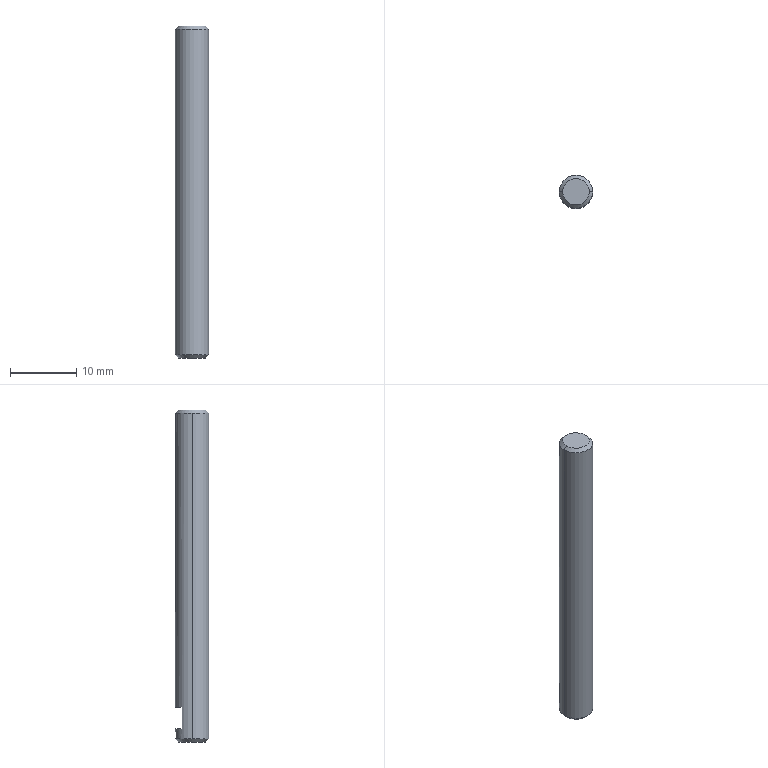Part | SolidWorks | features Chamfer 1, Extrusion 1, ICE 1 | 1 solid | 11 faces | box 5 x 5 x 50 mm | volume 969.137 mm3 | plane 5 | cone 4 | cylinder 2 | commonest cylinder face diameters 5 x2
STEP:
#1=CARTESIAN_POINT('',(2.,0.,25.));
#2=VERTEX_POINT('',#1);
#3=CARTESIAN_POINT('',(-2.,0.,25.));
#4=VERTEX_POINT('',#3);
#5=CARTESIAN_POINT('',(0.,0.,25.));
#6=DIRECTION('',(0.,0.,1.));
#7=DIRECTION('',(1.,0.,0.));
#8=AXIS2_PLACEMENT_3D('',#5,#6,#7);
#9=CIRCLE('',#8,2.);
#10=EDGE_CURVE('',#2,#4,#9,.T.);
#11=ORIENTED_EDGE('',*,*,#10,.F.);
#12=CARTESIAN_POINT('',(2.5,0.,24.5));
#13=VERTEX_POINT('',#12);
#14=CARTESIAN_POINT('',(2.,0.,25.));
#15=DIRECTION('',(0.7071,0.,-0.7071));
#16=VECTOR('',#15,1000.);
#17=LINE('',#14,#16);
#18=EDGE_CURVE('',#2,#13,#17,.T.);
#19=ORIENTED_EDGE('',*,*,#18,.T.);
#20=CARTESIAN_POINT('',(-2.5,0.,24.5));
#21=VERTEX_POINT('',#20);
#22=CARTESIAN_POINT('',(0.,0.,24.5));
#23=DIRECTION('',(0.,0.,-1.));
#24=DIRECTION('',(1.,0.,0.));
#25=AXIS2_PLACEMENT_3D('',#22,#23,#24);
#26=CIRCLE('',#25,2.5);
#27=EDGE_CURVE('',#21,#13,#26,.T.);
#28=ORIENTED_EDGE('',*,*,#27,.F.);
#29=CARTESIAN_POINT('',(-2.,0.,25.));
#30=DIRECTION('',(-0.7071,0.,-0.7071));
#31=VECTOR('',#30,1000.);
#32=LINE('',#29,#31);
#33=EDGE_CURVE('',#4,#21,#32,.T.);
#34=ORIENTED_EDGE('',*,*,#33,.F.);
#35=EDGE_LOOP('',(#11,#19,#28,#34));
#36=FACE_OUTER_BOUND('',#35,.T.);
#37=CARTESIAN_POINT('',(0.,0.,25.));
#38=DIRECTION('',(0.,0.,-1.));
#39=DIRECTION('',(-1.,0.,0.));
#40=AXIS2_PLACEMENT_3D('',#37,#38,#39);
#41=CONICAL_SURFACE('',#40,2.,0.7854);
#42=ADVANCED_FACE('',(#36),#41,.T.);
#43=CARTESIAN_POINT('',(-2.,0.,-25.));
#44=VERTEX_POINT('',#43);
#45=CARTESIAN_POINT('',(2.,0.,-25.));
#46=VERTEX_POINT('',#45);
#47=CARTESIAN_POINT('',(0.,0.,-25.));
#48=DIRECTION('',(0.,0.,-1.));
#49=DIRECTION('',(1.,0.,0.));
#50=AXIS2_PLACEMENT_3D('',#47,#48,#49);
#51=CIRCLE('',#50,2.);
#52=EDGE_CURVE('',#44,#46,#51,.T.);
#53=ORIENTED_EDGE('',*,*,#52,.F.);
#54=CARTESIAN_POINT('',(-2.5,0.,-24.5));
#55=VERTEX_POINT('',#54);
#56=CARTESIAN_POINT('',(-2.5,0.,-24.5));
#57=DIRECTION('',(-0.7071,0.,0.7071));
#58=VECTOR('',#57,1000.);
#59=LINE('',#56,#58);
#60=EDGE_CURVE('',#44,#55,#59,.T.);
#61=ORIENTED_EDGE('',*,*,#60,.T.);
#62=CARTESIAN_POINT('',(2.5,0.,-24.5));
#63=VERTEX_POINT('',#62);
#64=CARTESIAN_POINT('',(0.,0.,-24.5));
#65=DIRECTION('',(0.,0.,1.));
#66=DIRECTION('',(1.,0.,0.));
#67=AXIS2_PLACEMENT_3D('',#64,#65,#66);
#68=CIRCLE('',#67,2.5);
#69=EDGE_CURVE('',#63,#55,#68,.T.);
#70=ORIENTED_EDGE('',*,*,#69,.F.);
#71=CARTESIAN_POINT('',(2.5,0.,-24.5));
#72=DIRECTION('',(0.7071,0.,0.7071));
#73=VECTOR('',#72,1000.);
#74=LINE('',#71,#73);
#75=EDGE_CURVE('',#46,#63,#74,.T.);
#76=ORIENTED_EDGE('',*,*,#75,.F.);
#77=EDGE_LOOP('',(#53,#61,#70,#76));
#78=FACE_OUTER_BOUND('',#77,.T.);
#79=CARTESIAN_POINT('',(0.,0.,-24.5));
#80=DIRECTION('',(0.,0.,1.));
#81=DIRECTION('',(1.,0.,0.));
#82=AXIS2_PLACEMENT_3D('',#79,#80,#81);
#83=CONICAL_SURFACE('',#82,2.5,0.7854);
#84=ADVANCED_FACE('',(#78),#83,.T.);
#85=CARTESIAN_POINT('',(-2.,1.5,-19.8));
#86=VERTEX_POINT('',#85);
#87=CARTESIAN_POINT('',(-2.,1.5,-23.));
#88=VERTEX_POINT('',#87);
#89=CARTESIAN_POINT('',(-2.,1.5,25.));
#90=DIRECTION('',(0.,0.,-1.));
#91=VECTOR('',#90,1000.);
#92=LINE('',#89,#91);
#93=EDGE_CURVE('',#86,#88,#92,.T.);
#94=ORIENTED_EDGE('',*,*,#93,.T.);
#95=CARTESIAN_POINT('',(2.,1.5,-23.));
#96=VERTEX_POINT('',#95);
#97=CARTESIAN_POINT('',(0.,0.,-23.));
#98=DIRECTION('',(0.,0.,-1.));
#99=DIRECTION('',(-1.,0.,0.));
#100=AXIS2_PLACEMENT_3D('',#97,#98,#99);
#101=CIRCLE('',#100,2.5);
#102=EDGE_CURVE('',#88,#96,#101,.T.);
#103=ORIENTED_EDGE('',*,*,#102,.T.);
#104=CARTESIAN_POINT('',(2.,1.5,-19.8));
#105=VERTEX_POINT('',#104);
#106=CARTESIAN_POINT('',(2.,1.5,25.));
#107=DIRECTION('',(0.,0.,1.));
#108=VECTOR('',#107,1000.);
#109=LINE('',#106,#108);
#110=EDGE_CURVE('',#96,#105,#109,.T.);
#111=ORIENTED_EDGE('',*,*,#110,.T.);
#112=CARTESIAN_POINT('',(0.,0.,-19.8));
#113=DIRECTION('',(0.,0.,1.));
#114=DIRECTION('',(0.,-1.,0.));
#115=AXIS2_PLACEMENT_3D('',#112,#113,#114);
#116=CIRCLE('',#115,2.5);
#117=EDGE_CURVE('',#105,#86,#116,.T.);
#118=ORIENTED_EDGE('',*,*,#117,.T.);
#119=EDGE_LOOP('',(#94,#103,#111,#118));
#120=FACE_BOUND('',#119,.T.);
#121=ORIENTED_EDGE('',*,*,#27,.T.);
#122=CARTESIAN_POINT('',(2.5,0.,25.));
#123=DIRECTION('',(0.,0.,-1.));
#124=VECTOR('',#123,1000.);
#125=LINE('',#122,#124);
#126=EDGE_CURVE('',#13,#63,#125,.T.);
#127=ORIENTED_EDGE('',*,*,#126,.T.);
#128=ORIENTED_EDGE('',*,*,#69,.T.);
#129=CARTESIAN_POINT('',(-2.5,0.,25.));
#130=DIRECTION('',(0.,0.,-1.));
#131=VECTOR('',#130,1000.);
#132=LINE('',#129,#131);
#133=EDGE_CURVE('',#21,#55,#132,.T.);
#134=ORIENTED_EDGE('',*,*,#133,.F.);
#135=EDGE_LOOP('',(#121,#127,#128,#134));
#136=FACE_OUTER_BOUND('',#135,.T.);
#137=CARTESIAN_POINT('',(0.,0.,25.));
#138=DIRECTION('',(0.,0.,-1.));
#139=DIRECTION('',(-1.,0.,0.));
#140=AXIS2_PLACEMENT_3D('',#137,#138,#139);
#141=CYLINDRICAL_SURFACE('',#140,2.5);
#142=ADVANCED_FACE('',(#120,#136),#141,.T.);
#143=ORIENTED_EDGE('',*,*,#126,.F.);
#144=CARTESIAN_POINT('',(0.,0.,24.5));
#145=DIRECTION('',(0.,0.,-1.));
#146=DIRECTION('',(1.,0.,0.));
#147=AXIS2_PLACEMENT_3D('',#144,#145,#146);
#148=CIRCLE('',#147,2.5);
#149=EDGE_CURVE('',#13,#21,#148,.T.);
#150=ORIENTED_EDGE('',*,*,#149,.T.);
#151=ORIENTED_EDGE('',*,*,#133,.T.);
#152=CARTESIAN_POINT('',(0.,0.,-24.5));
#153=DIRECTION('',(0.,0.,1.));
#154=DIRECTION('',(1.,0.,0.));
#155=AXIS2_PLACEMENT_3D('',#152,#153,#154);
#156=CIRCLE('',#155,2.5);
#157=EDGE_CURVE('',#55,#63,#156,.T.);
#158=ORIENTED_EDGE('',*,*,#157,.T.);
#159=EDGE_LOOP('',(#143,#150,#151,#158));
#160=FACE_OUTER_BOUND('',#159,.T.);
#161=CARTESIAN_POINT('',(0.,0.,25.));
#162=DIRECTION('',(0.,0.,-1.));
#163=DIRECTION('',(-1.,0.,0.));
#164=AXIS2_PLACEMENT_3D('',#161,#162,#163);
#165=CYLINDRICAL_SURFACE('',#164,2.5);
#166=ADVANCED_FACE('',(#160),#165,.T.);
#167=CARTESIAN_POINT('',(0.,0.,25.));
#168=DIRECTION('',(0.,0.,1.));
#169=DIRECTION('',(1.,0.,0.));
#170=AXIS2_PLACEMENT_3D('',#167,#168,#169);
#171=CIRCLE('',#170,2.);
#172=EDGE_CURVE('',#4,#2,#171,.T.);
#173=ORIENTED_EDGE('',*,*,#172,.T.);
#174=ORIENTED_EDGE('',*,*,#10,.T.);
#175=EDGE_LOOP('',(#173,#174));
#176=FACE_OUTER_BOUND('',#175,.T.);
#177=CARTESIAN_POINT('',(0.,0.,25.));
#178=DIRECTION('',(0.,0.,1.));
#179=DIRECTION('',(1.,0.,0.));
#180=AXIS2_PLACEMENT_3D('',#177,#178,#179);
#181=PLANE('',#180);
#182=ADVANCED_FACE('',(#176),#181,.T.);
#183=CARTESIAN_POINT('',(0.,0.,-25.));
#184=DIRECTION('',(0.,0.,-1.));
#185=DIRECTION('',(1.,0.,0.));
#186=AXIS2_PLACEMENT_3D('',#183,#184,#185);
#187=CIRCLE('',#186,2.);
#188=EDGE_CURVE('',#46,#44,#187,.T.);
#189=ORIENTED_EDGE('',*,*,#188,.T.);
#190=ORIENTED_EDGE('',*,*,#52,.T.);
#191=EDGE_LOOP('',(#189,#190));
#192=FACE_OUTER_BOUND('',#191,.T.);
#193=CARTESIAN_POINT('',(0.,0.,-25.));
#194=DIRECTION('',(0.,0.,1.));
#195=DIRECTION('',(1.,0.,0.));
#196=AXIS2_PLACEMENT_3D('',#193,#194,#195);
#197=PLANE('',#196);
#198=ADVANCED_FACE('',(#192),#197,.F.);
#199=ORIENTED_EDGE('',*,*,#60,.F.);
#200=ORIENTED_EDGE('',*,*,#188,.F.);
#201=ORIENTED_EDGE('',*,*,#75,.T.);
#202=ORIENTED_EDGE('',*,*,#157,.F.);
#203=EDGE_LOOP('',(#199,#200,#201,#202));
#204=FACE_OUTER_BOUND('',#203,.T.);
#205=CARTESIAN_POINT('',(0.,0.,-24.5));
#206=DIRECTION('',(0.,0.,1.));
#207=DIRECTION('',(1.,0.,0.));
#208=AXIS2_PLACEMENT_3D('',#205,#206,#207);
#209=CONICAL_SURFACE('',#208,2.5,0.7854);
#210=ADVANCED_FACE('',(#204),#209,.T.);
#211=ORIENTED_EDGE('',*,*,#18,.F.);
#212=ORIENTED_EDGE('',*,*,#172,.F.);
#213=ORIENTED_EDGE('',*,*,#33,.T.);
#214=ORIENTED_EDGE('',*,*,#149,.F.);
#215=EDGE_LOOP('',(#211,#212,#213,#214));
#216=FACE_OUTER_BOUND('',#215,.T.);
#217=CARTESIAN_POINT('',(0.,0.,25.));
#218=DIRECTION('',(0.,0.,-1.));
#219=DIRECTION('',(-1.,0.,0.));
#220=AXIS2_PLACEMENT_3D('',#217,#218,#219);
#221=CONICAL_SURFACE('',#220,2.,0.7854);
#222=ADVANCED_FACE('',(#216),#221,.T.);
#223=CARTESIAN_POINT('',(-2.5,1.5,-23.));
#224=DIRECTION('',(1.,0.,0.));
#225=VECTOR('',#224,1000.);
#226=LINE('',#223,#225);
#227=EDGE_CURVE('',#88,#96,#226,.T.);
#228=ORIENTED_EDGE('',*,*,#227,.T.);
#229=ORIENTED_EDGE('',*,*,#102,.F.);
#230=EDGE_LOOP('',(#228,#229));
#231=FACE_OUTER_BOUND('',#230,.T.);
#232=CARTESIAN_POINT('',(-2.5,5.025,-23.));
#233=DIRECTION('',(0.,0.,-1.));
#234=DIRECTION('',(-1.,0.,0.));
#235=AXIS2_PLACEMENT_3D('',#232,#233,#234);
#236=PLANE('',#235);
#237=ADVANCED_FACE('',(#231),#236,.F.);
#238=CARTESIAN_POINT('',(-2.5,1.5,-19.8));
#239=DIRECTION('',(1.,0.,0.));
#240=VECTOR('',#239,1000.);
#241=LINE('',#238,#240);
#242=EDGE_CURVE('',#86,#105,#241,.T.);
#243=ORIENTED_EDGE('',*,*,#242,.T.);
#244=ORIENTED_EDGE('',*,*,#110,.F.);
#245=ORIENTED_EDGE('',*,*,#227,.F.);
#246=ORIENTED_EDGE('',*,*,#93,.F.);
#247=EDGE_LOOP('',(#243,#244,#245,#246));
#248=FACE_OUTER_BOUND('',#247,.T.);
#249=CARTESIAN_POINT('',(-2.5,1.5,-23.));
#250=DIRECTION('',(0.,-1.,0.));
#251=DIRECTION('',(0.,0.,-1.));
#252=AXIS2_PLACEMENT_3D('',#249,#250,#251);
#253=PLANE('',#252);
#254=ADVANCED_FACE('',(#248),#253,.F.);
#255=ORIENTED_EDGE('',*,*,#242,.F.);
#256=ORIENTED_EDGE('',*,*,#117,.F.);
#257=EDGE_LOOP('',(#255,#256));
#258=FACE_OUTER_BOUND('',#257,.T.);
#259=CARTESIAN_POINT('',(-2.5,5.025,-19.8));
#260=DIRECTION('',(0.,0.,1.));
#261=DIRECTION('',(0.,-1.,0.));
#262=AXIS2_PLACEMENT_3D('',#259,#260,#261);
#263=PLANE('',#262);
#264=ADVANCED_FACE('',(#258),#263,.F.);
#265=CLOSED_SHELL('',(#42,#84,#142,#166,#182,#198,#210,#222,#237,#254,#264));
#266=MANIFOLD_SOLID_BREP('',#265);
#267=CARTESIAN_POINT('',(0.,0.,0.));
#268=DIRECTION('',(0.,0.,1.));
#269=DIRECTION('',(1.,0.,0.));
#270=AXIS2_PLACEMENT_3D('',#267,#268,#269);
#271=(LENGTH_UNIT()NAMED_UNIT(*)SI_UNIT(.MILLI.,.METRE.));
#272=UNCERTAINTY_MEASURE_WITH_UNIT(LENGTH_MEASURE(0.00001),#271,'','');
#273=(NAMED_UNIT(*)PLANE_ANGLE_UNIT()SI_UNIT($,.RADIAN.));
#274=(NAMED_UNIT(*)SI_UNIT($,.STERADIAN.)SOLID_ANGLE_UNIT());
#275=(GEOMETRIC_REPRESENTATION_CONTEXT(3)GLOBAL_UNCERTAINTY_ASSIGNED_CONTEXT((#272))GLOBAL_UNIT_ASSIGNED_CONTEXT((#271,#273,#274))REPRESENTATION_CONTEXT('',''));
#276=ADVANCED_BREP_SHAPE_REPRESENTATION('',(#266,#270),#275);